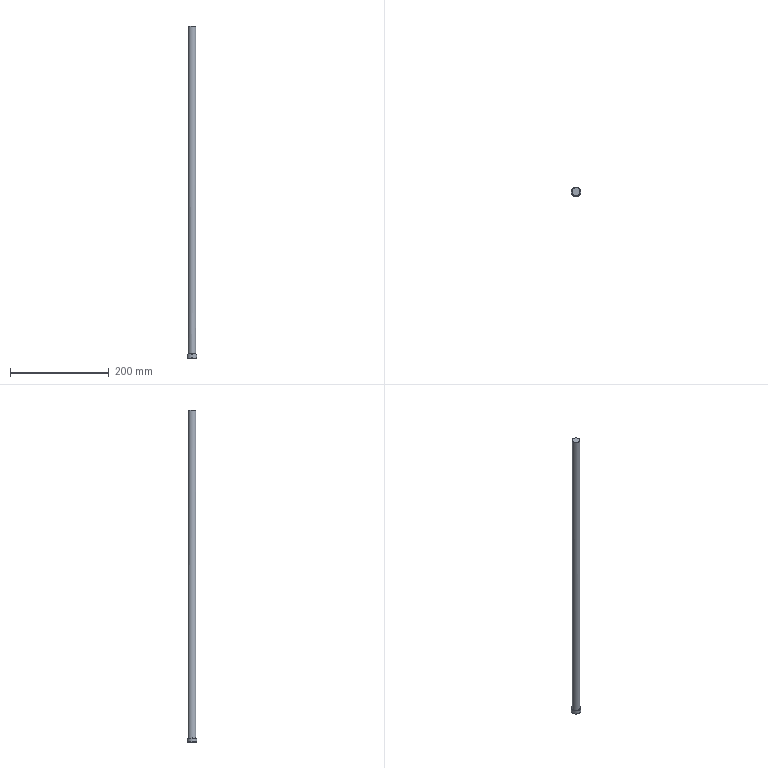Part | STEP file | solid 121 | 1 solid | 47 faces | box 20 x 20 x 674.011 mm | volume 136324 mm3 | other 21 | plane 20 | cylinder 2 | cone 2 | spline 1 | torus 1 | commonest cylinder face diameters 16 x1 20 x1